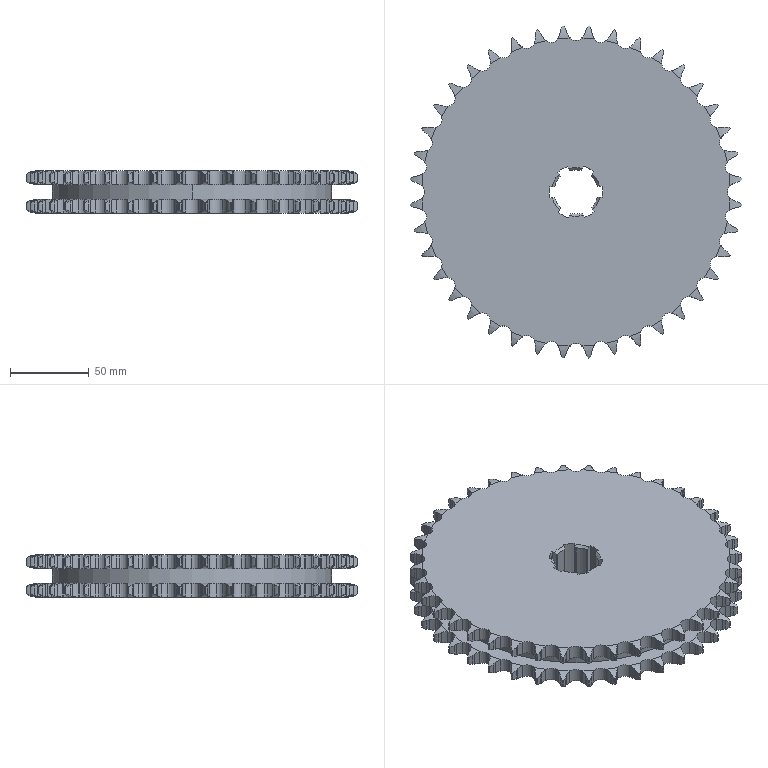Part | SolidWorks | features BaseBody 1 | 1 solid | 909 faces | box 211.077 x 210.652 x 26.852 mm | volume 750377 mm3 | cylinder 548 | plane 188 | spline 160 | cone 13 | commonest cylinder face diameters 16.487 x168 26.518 x168 10.262 x102 211.236 x80 0.2 x15 28 x7